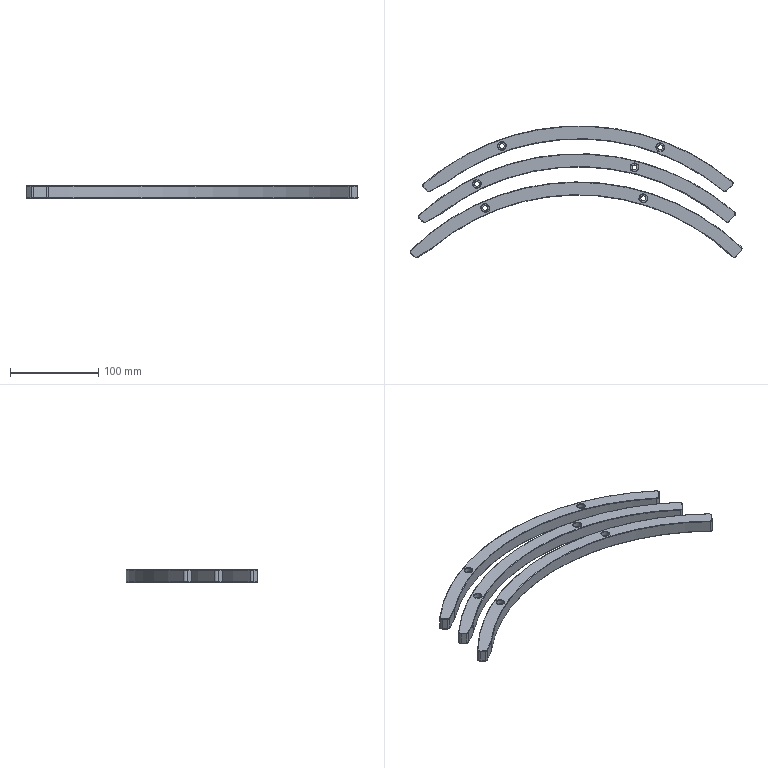CAM job | NX | 3-axis milling, drilling | part box 376.065 x 149.521 x 14 mm | stock box 381.08 x 154.541 x 15 mm
Tools:
number,name,description,diameter,corner_radius,flute_length,length,flutes
6,D6,平底铣刀-粗,6.0,0.0,25.0,75.0,2
9,D10,平底铣刀-粗,10.0,0.0,35.0,75.0,2
18,D3-J,平底铣刀-精,3.0,0.0,50.0,75.0,2
7,D6-J,平底铣刀-精,6.0,0.0,25.0,75.0,2
19,D6R0.5,圆鼻刀-粗,6.0,0.5,50.0,75.0,2
1,D80R0.8飞刀,圆鼻刀-粗,80.0,0.8,50.0,75.0,2
1,D80R0.8飞刀-J,圆鼻刀-精,80.0,0.8,50.0,75.0,2
2,D6倒角刀,倒角刀,6.0,0.0,3.0,25.0,2
17,钻头5.5,Twist Drill 5 mm,5.5,0.0,52.0,54.0,2
Operations:
program,operation,operation_type,tool,method,geometry_group,spindle_rpm,surface_speed,feed_per_tooth,feed_cut,feed_plunge,cut_length_mm,path_length_mm,cut_time_min,machine_time_min
A,底壁铣飞面开粗_COPY,VolumeBased25DMillingOperation,D80R0.8飞刀,分层开粗-切深K-步距G,W-A,2800.0,703.696,0.5357,3000.0,100.0,2777.131,3263.663,0.9257,0.9744
A,底壁铣飞面精光_COPY,VolumeBased25DMillingOperation,D80R0.8飞刀-J,侧刃精光-切深K-步距G,W-A,4000.0,1005.28,0.125,1000.0,100.0,1387.855,1423.855,1.388,1.391
A,打点,Operation,D6倒角刀,METHOD,W-A,3000.0,56.549,0.0333,200.0,0.0,15.0,399.377,0.075,0.1134
A,打孔,Operation,钻头5.5,METHOD,W-A,2600.0,44.925,0.0231,120.0,0.0,88.2,545.777,0.735,0.7808
A,孔粗_1,CylinderMilling,D6,METHOD,W-A,6000.0,113.097,0.1667,2000.0,100.0,954.671,1571.429,0.4773,0.539
A,外形粗_2,VolumeBased25DMillingOperation,D10,METHOD,W-A,6000.0,188.0,0.25,4000.0,80.0,74960.853,75227.167,18.74,18.767
A,孔侧_1,CylinderMilling,D6-J,METHOD,W-A,6000.0,113.097,0.05,600.0,100.0,80.553,732.111,0.1343,0.1994
A,底壁铣螺旋精光-中_COPY,VolumeBased25DMillingOperation,D3-J,螺旋精光-切深K-步距G,W-A,8000.0,75.396,0.0375,600.0,100.0,1434.325,2107.314,2.39,2.458
A,等高精光往复爬面_COPY,ZLevelMilling,D6R0.5,等高爬面-切深K-步距G,W-A,8000.0,150.796,0.3125,5000.0,100.0,36819.148,36958.763,7.364,7.378
A,铣倒角_1,PlanarMilling,D6倒角刀,METHOD,W-A,6000.0,113.097,0.05,600.0,100.0,140.515,729.205,0.2342,0.2931
A,外形半精_2,VolumeBased25DMillingOperation,D6-J,METHOD,W-A,6000.0,113.0,0.0833,1000.0,100.0,4948.058,5389.827,4.948,4.992
A,外形精_2,VolumeBased25DMillingOperation,D6-J,METHOD,W-A,6000.0,113.0,0.0833,1000.0,100.0,2473.429,2751.907,2.473,2.501